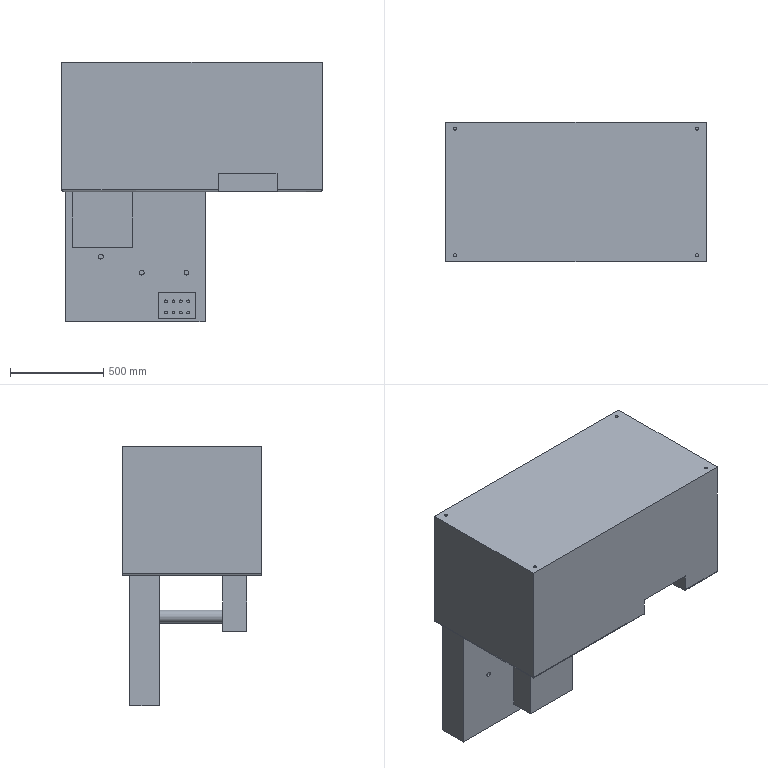Part | STEP file | 1 solid | 94 faces | box 1400 x 750 x 1396 mm | volume 760190191 mm3 | plane 48 | cylinder 46 | commonest cylinder face diameters 15 x16 16 x8 20 x6 25 x6 11.633 x2 12.618 x2